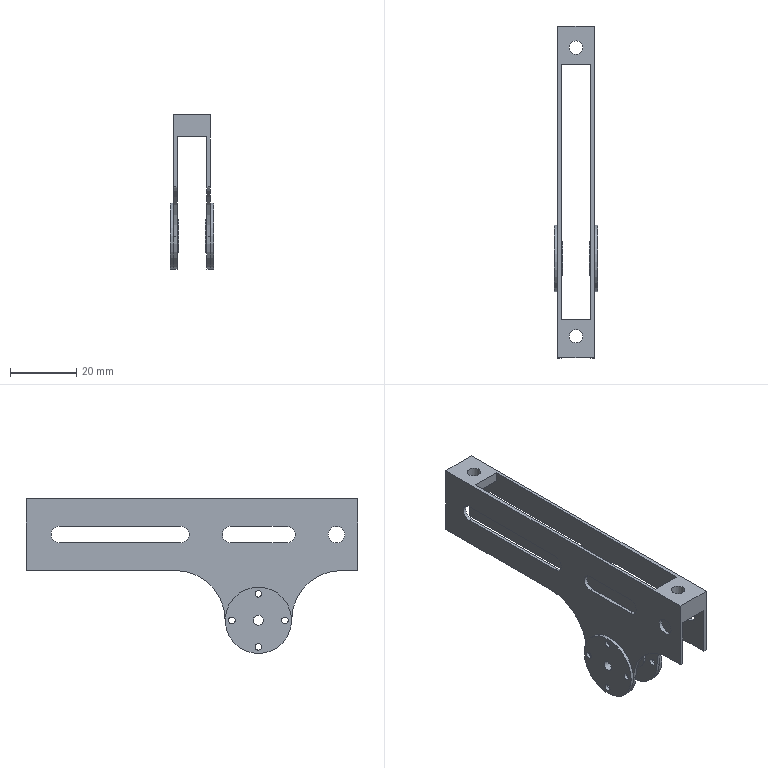Part | STEP file | 1-28.10 | 3 solids | 75 faces | box 13 x 100 x 46.631 mm | volume 6044 mm3 | cylinder 42 | plane 33 | commonest cylinder face diameters 2 x16 5 x10 10 x4 20 x4 30 x4 3 x2